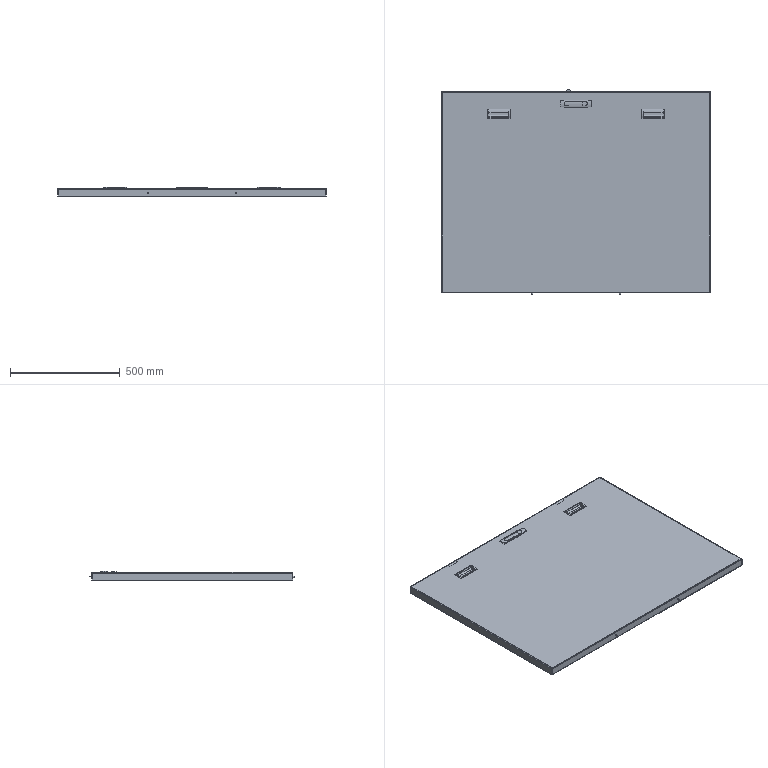Part | SolidWorks | 8 solids | 520 faces | box 1225 x 936.5 x 44 mm | volume 2159359 mm3 | plane 248 | cylinder 194 | spline 46 | cone 26 | torus 6 | commonest cylinder face diameters 10 x27 2 x20 8.136 x15 7 x13 4 x12 6.6 x12